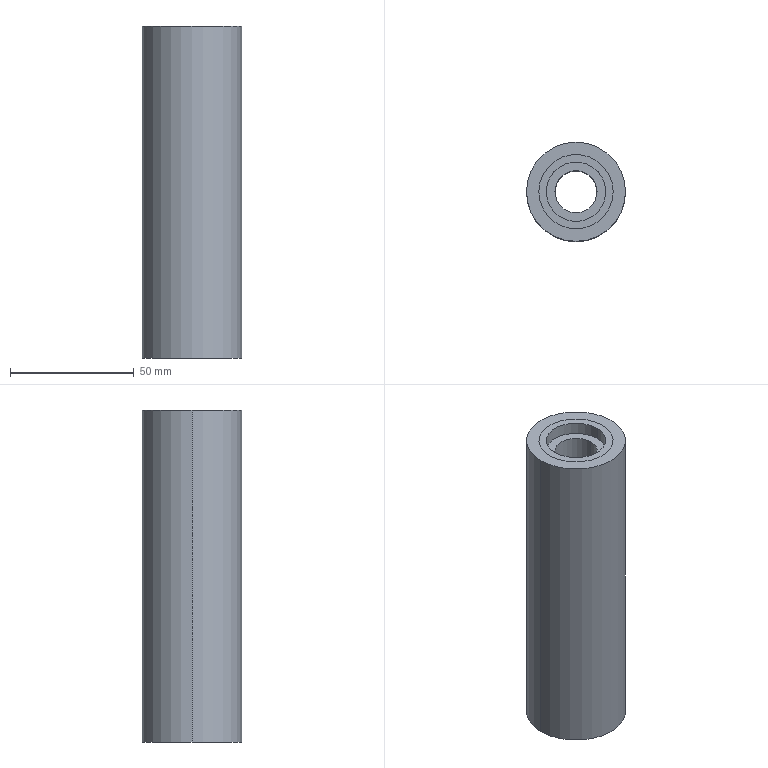Part | STEP file | MT-COMBO-119-S016 | 2 solids | 18 faces | box 40 x 40 x 134 mm | volume 135720 mm3 | cylinder 12 | plane 6 | commonest cylinder face diameters 24 x4 30 x4 17 x2 40 x2
STEP:
#1=CARTESIAN_POINT('',(12.,0.,62.));
#2=VERTEX_POINT('',#1);
#3=CARTESIAN_POINT('',(-12.,0.,62.));
#4=VERTEX_POINT('',#3);
#5=CARTESIAN_POINT('',(0.,0.,62.));
#6=DIRECTION('',(0.,0.,1.));
#7=DIRECTION('',(1.,0.,0.));
#8=AXIS2_PLACEMENT_3D('',#5,#6,#7);
#9=CIRCLE('',#8,12.);
#10=EDGE_CURVE('',#2,#4,#9,.T.);
#11=ORIENTED_EDGE('',*,*,#10,.F.);
#12=CARTESIAN_POINT('',(12.,0.,67.));
#13=VERTEX_POINT('',#12);
#14=CARTESIAN_POINT('',(12.,0.,62.));
#15=DIRECTION('',(0.,0.,1.));
#16=VECTOR('',#15,1000.);
#17=LINE('',#14,#16);
#18=EDGE_CURVE('',#2,#13,#17,.T.);
#19=ORIENTED_EDGE('',*,*,#18,.T.);
#20=CARTESIAN_POINT('',(-12.,0.,67.));
#21=VERTEX_POINT('',#20);
#22=CARTESIAN_POINT('',(0.,0.,67.));
#23=DIRECTION('',(0.,0.,1.));
#24=DIRECTION('',(1.,0.,0.));
#25=AXIS2_PLACEMENT_3D('',#22,#23,#24);
#26=CIRCLE('',#25,12.);
#27=EDGE_CURVE('',#13,#21,#26,.T.);
#28=ORIENTED_EDGE('',*,*,#27,.T.);
#29=CARTESIAN_POINT('',(-12.,0.,62.));
#30=DIRECTION('',(0.,0.,1.));
#31=VECTOR('',#30,1000.);
#32=LINE('',#29,#31);
#33=EDGE_CURVE('',#4,#21,#32,.T.);
#34=ORIENTED_EDGE('',*,*,#33,.F.);
#35=EDGE_LOOP('',(#11,#19,#28,#34));
#36=FACE_OUTER_BOUND('',#35,.T.);
#37=CARTESIAN_POINT('',(0.,0.,62.));
#38=DIRECTION('',(0.,0.,1.));
#39=DIRECTION('',(-1.,0.,0.));
#40=AXIS2_PLACEMENT_3D('',#37,#38,#39);
#41=CYLINDRICAL_SURFACE('',#40,12.);
#42=ADVANCED_FACE('',(#36),#41,.F.);
#43=CARTESIAN_POINT('',(12.,0.,-62.));
#44=VERTEX_POINT('',#43);
#45=CARTESIAN_POINT('',(-12.,0.,-62.));
#46=VERTEX_POINT('',#45);
#47=CARTESIAN_POINT('',(0.,0.,-62.));
#48=DIRECTION('',(0.,0.,1.));
#49=DIRECTION('',(1.,0.,0.));
#50=AXIS2_PLACEMENT_3D('',#47,#48,#49);
#51=CIRCLE('',#50,12.);
#52=EDGE_CURVE('',#44,#46,#51,.T.);
#53=ORIENTED_EDGE('',*,*,#52,.T.);
#54=CARTESIAN_POINT('',(-12.,0.,-67.));
#55=VERTEX_POINT('',#54);
#56=CARTESIAN_POINT('',(-12.,0.,-62.));
#57=DIRECTION('',(0.,0.,-1.));
#58=VECTOR('',#57,1000.);
#59=LINE('',#56,#58);
#60=EDGE_CURVE('',#46,#55,#59,.T.);
#61=ORIENTED_EDGE('',*,*,#60,.T.);
#62=CARTESIAN_POINT('',(12.,0.,-67.));
#63=VERTEX_POINT('',#62);
#64=CARTESIAN_POINT('',(0.,0.,-67.));
#65=DIRECTION('',(0.,0.,1.));
#66=DIRECTION('',(1.,0.,0.));
#67=AXIS2_PLACEMENT_3D('',#64,#65,#66);
#68=CIRCLE('',#67,12.);
#69=EDGE_CURVE('',#63,#55,#68,.T.);
#70=ORIENTED_EDGE('',*,*,#69,.F.);
#71=CARTESIAN_POINT('',(12.,0.,-62.));
#72=DIRECTION('',(0.,0.,-1.));
#73=VECTOR('',#72,1000.);
#74=LINE('',#71,#73);
#75=EDGE_CURVE('',#44,#63,#74,.T.);
#76=ORIENTED_EDGE('',*,*,#75,.F.);
#77=EDGE_LOOP('',(#53,#61,#70,#76));
#78=FACE_OUTER_BOUND('',#77,.T.);
#79=CARTESIAN_POINT('',(0.,0.,-62.));
#80=DIRECTION('',(0.,0.,-1.));
#81=DIRECTION('',(1.,0.,0.));
#82=AXIS2_PLACEMENT_3D('',#79,#80,#81);
#83=CYLINDRICAL_SURFACE('',#82,12.);
#84=ADVANCED_FACE('',(#78),#83,.F.);
#85=CARTESIAN_POINT('',(-15.,0.,-67.));
#86=VERTEX_POINT('',#85);
#87=CARTESIAN_POINT('',(15.,0.,-67.));
#88=VERTEX_POINT('',#87);
#89=CARTESIAN_POINT('',(0.,0.,-67.));
#90=DIRECTION('',(0.,0.,1.));
#91=DIRECTION('',(1.,0.,0.));
#92=AXIS2_PLACEMENT_3D('',#89,#90,#91);
#93=CIRCLE('',#92,15.);
#94=EDGE_CURVE('',#86,#88,#93,.T.);
#95=ORIENTED_EDGE('',*,*,#94,.T.);
#96=CARTESIAN_POINT('',(15.,0.,67.));
#97=VERTEX_POINT('',#96);
#98=CARTESIAN_POINT('',(15.,0.,-67.));
#99=DIRECTION('',(0.,0.,1.));
#100=VECTOR('',#99,1000.);
#101=LINE('',#98,#100);
#102=EDGE_CURVE('',#88,#97,#101,.T.);
#103=ORIENTED_EDGE('',*,*,#102,.T.);
#104=CARTESIAN_POINT('',(-15.,0.,67.));
#105=VERTEX_POINT('',#104);
#106=CARTESIAN_POINT('',(0.,0.,67.));
#107=DIRECTION('',(0.,0.,1.));
#108=DIRECTION('',(1.,0.,0.));
#109=AXIS2_PLACEMENT_3D('',#106,#107,#108);
#110=CIRCLE('',#109,15.);
#111=EDGE_CURVE('',#105,#97,#110,.T.);
#112=ORIENTED_EDGE('',*,*,#111,.F.);
#113=CARTESIAN_POINT('',(-15.,0.,-67.));
#114=DIRECTION('',(0.,0.,1.));
#115=VECTOR('',#114,1000.);
#116=LINE('',#113,#115);
#117=EDGE_CURVE('',#86,#105,#116,.T.);
#118=ORIENTED_EDGE('',*,*,#117,.F.);
#119=EDGE_LOOP('',(#95,#103,#112,#118));
#120=FACE_OUTER_BOUND('',#119,.T.);
#121=CARTESIAN_POINT('',(0.,0.,-67.));
#122=DIRECTION('',(0.,0.,1.));
#123=DIRECTION('',(-1.,0.,0.));
#124=AXIS2_PLACEMENT_3D('',#121,#122,#123);
#125=CYLINDRICAL_SURFACE('',#124,15.);
#126=ADVANCED_FACE('',(#120),#125,.T.);
#127=CARTESIAN_POINT('',(8.5,0.,-62.));
#128=VERTEX_POINT('',#127);
#129=CARTESIAN_POINT('',(-8.5,0.,-62.));
#130=VERTEX_POINT('',#129);
#131=CARTESIAN_POINT('',(0.,0.,-62.));
#132=DIRECTION('',(0.,0.,1.));
#133=DIRECTION('',(1.,0.,0.));
#134=AXIS2_PLACEMENT_3D('',#131,#132,#133);
#135=CIRCLE('',#134,8.5);
#136=EDGE_CURVE('',#128,#130,#135,.T.);
#137=ORIENTED_EDGE('',*,*,#136,.F.);
#138=CARTESIAN_POINT('',(8.5,0.,62.));
#139=VERTEX_POINT('',#138);
#140=CARTESIAN_POINT('',(8.5,0.,-67.));
#141=DIRECTION('',(0.,0.,1.));
#142=VECTOR('',#141,1000.);
#143=LINE('',#140,#142);
#144=EDGE_CURVE('',#128,#139,#143,.T.);
#145=ORIENTED_EDGE('',*,*,#144,.T.);
#146=CARTESIAN_POINT('',(-8.5,0.,62.));
#147=VERTEX_POINT('',#146);
#148=CARTESIAN_POINT('',(0.,0.,62.));
#149=DIRECTION('',(0.,0.,-1.));
#150=DIRECTION('',(-1.,0.,0.));
#151=AXIS2_PLACEMENT_3D('',#148,#149,#150);
#152=CIRCLE('',#151,8.5);
#153=EDGE_CURVE('',#147,#139,#152,.T.);
#154=ORIENTED_EDGE('',*,*,#153,.F.);
#155=CARTESIAN_POINT('',(-8.5,0.,-67.));
#156=DIRECTION('',(0.,0.,1.));
#157=VECTOR('',#156,1000.);
#158=LINE('',#155,#157);
#159=EDGE_CURVE('',#130,#147,#158,.T.);
#160=ORIENTED_EDGE('',*,*,#159,.F.);
#161=EDGE_LOOP('',(#137,#145,#154,#160));
#162=FACE_OUTER_BOUND('',#161,.T.);
#163=CARTESIAN_POINT('',(0.,0.,-67.));
#164=DIRECTION('',(0.,0.,1.));
#165=DIRECTION('',(-1.,0.,0.));
#166=AXIS2_PLACEMENT_3D('',#163,#164,#165);
#167=CYLINDRICAL_SURFACE('',#166,8.5);
#168=ADVANCED_FACE('',(#162),#167,.F.);
#169=ORIENTED_EDGE('',*,*,#144,.F.);
#170=CARTESIAN_POINT('',(0.,0.,-62.));
#171=DIRECTION('',(0.,0.,1.));
#172=DIRECTION('',(1.,0.,0.));
#173=AXIS2_PLACEMENT_3D('',#170,#171,#172);
#174=CIRCLE('',#173,8.5);
#175=EDGE_CURVE('',#130,#128,#174,.T.);
#176=ORIENTED_EDGE('',*,*,#175,.F.);
#177=ORIENTED_EDGE('',*,*,#159,.T.);
#178=CARTESIAN_POINT('',(0.,0.,62.));
#179=DIRECTION('',(0.,0.,-1.));
#180=DIRECTION('',(-1.,0.,0.));
#181=AXIS2_PLACEMENT_3D('',#178,#179,#180);
#182=CIRCLE('',#181,8.5);
#183=EDGE_CURVE('',#139,#147,#182,.T.);
#184=ORIENTED_EDGE('',*,*,#183,.F.);
#185=EDGE_LOOP('',(#169,#176,#177,#184));
#186=FACE_OUTER_BOUND('',#185,.T.);
#187=CARTESIAN_POINT('',(0.,0.,-67.));
#188=DIRECTION('',(0.,0.,1.));
#189=DIRECTION('',(-1.,0.,0.));
#190=AXIS2_PLACEMENT_3D('',#187,#188,#189);
#191=CYLINDRICAL_SURFACE('',#190,8.5);
#192=ADVANCED_FACE('',(#186),#191,.F.);
#193=ORIENTED_EDGE('',*,*,#69,.T.);
#194=CARTESIAN_POINT('',(0.,0.,-67.));
#195=DIRECTION('',(0.,0.,1.));
#196=DIRECTION('',(1.,0.,0.));
#197=AXIS2_PLACEMENT_3D('',#194,#195,#196);
#198=CIRCLE('',#197,12.);
#199=EDGE_CURVE('',#55,#63,#198,.T.);
#200=ORIENTED_EDGE('',*,*,#199,.T.);
#201=EDGE_LOOP('',(#193,#200));
#202=FACE_BOUND('',#201,.T.);
#203=ORIENTED_EDGE('',*,*,#94,.F.);
#204=CARTESIAN_POINT('',(0.,0.,-67.));
#205=DIRECTION('',(0.,0.,1.));
#206=DIRECTION('',(1.,0.,0.));
#207=AXIS2_PLACEMENT_3D('',#204,#205,#206);
#208=CIRCLE('',#207,15.);
#209=EDGE_CURVE('',#88,#86,#208,.T.);
#210=ORIENTED_EDGE('',*,*,#209,.F.);
#211=EDGE_LOOP('',(#203,#210));
#212=FACE_OUTER_BOUND('',#211,.T.);
#213=CARTESIAN_POINT('',(0.,0.,-67.));
#214=DIRECTION('',(0.,0.,-1.));
#215=DIRECTION('',(1.,0.,0.));
#216=AXIS2_PLACEMENT_3D('',#213,#214,#215);
#217=PLANE('',#216);
#218=ADVANCED_FACE('',(#202,#212),#217,.T.);
#219=CARTESIAN_POINT('',(0.,0.,67.));
#220=DIRECTION('',(0.,0.,1.));
#221=DIRECTION('',(1.,0.,0.));
#222=AXIS2_PLACEMENT_3D('',#219,#220,#221);
#223=CIRCLE('',#222,12.);
#224=EDGE_CURVE('',#21,#13,#223,.T.);
#225=ORIENTED_EDGE('',*,*,#224,.F.);
#226=ORIENTED_EDGE('',*,*,#27,.F.);
#227=EDGE_LOOP('',(#225,#226));
#228=FACE_BOUND('',#227,.T.);
#229=ORIENTED_EDGE('',*,*,#111,.T.);
#230=CARTESIAN_POINT('',(0.,0.,67.));
#231=DIRECTION('',(0.,0.,1.));
#232=DIRECTION('',(1.,0.,0.));
#233=AXIS2_PLACEMENT_3D('',#230,#231,#232);
#234=CIRCLE('',#233,15.);
#235=EDGE_CURVE('',#97,#105,#234,.T.);
#236=ORIENTED_EDGE('',*,*,#235,.T.);
#237=EDGE_LOOP('',(#229,#236));
#238=FACE_OUTER_BOUND('',#237,.T.);
#239=CARTESIAN_POINT('',(0.,0.,67.));
#240=DIRECTION('',(0.,0.,-1.));
#241=DIRECTION('',(1.,0.,0.));
#242=AXIS2_PLACEMENT_3D('',#239,#240,#241);
#243=PLANE('',#242);
#244=ADVANCED_FACE('',(#228,#238),#243,.F.);
#245=ORIENTED_EDGE('',*,*,#102,.F.);
#246=ORIENTED_EDGE('',*,*,#209,.T.);
#247=ORIENTED_EDGE('',*,*,#117,.T.);
#248=ORIENTED_EDGE('',*,*,#235,.F.);
#249=EDGE_LOOP('',(#245,#246,#247,#248));
#250=FACE_OUTER_BOUND('',#249,.T.);
#251=CARTESIAN_POINT('',(0.,0.,-67.));
#252=DIRECTION('',(0.,0.,1.));
#253=DIRECTION('',(-1.,0.,0.));
#254=AXIS2_PLACEMENT_3D('',#251,#252,#253);
#255=CYLINDRICAL_SURFACE('',#254,15.);
#256=ADVANCED_FACE('',(#250),#255,.T.);
#257=ORIENTED_EDGE('',*,*,#60,.F.);
#258=CARTESIAN_POINT('',(0.,0.,-62.));
#259=DIRECTION('',(0.,0.,1.));
#260=DIRECTION('',(1.,0.,0.));
#261=AXIS2_PLACEMENT_3D('',#258,#259,#260);
#262=CIRCLE('',#261,12.);
#263=EDGE_CURVE('',#46,#44,#262,.T.);
#264=ORIENTED_EDGE('',*,*,#263,.T.);
#265=ORIENTED_EDGE('',*,*,#75,.T.);
#266=ORIENTED_EDGE('',*,*,#199,.F.);
#267=EDGE_LOOP('',(#257,#264,#265,#266));
#268=FACE_OUTER_BOUND('',#267,.T.);
#269=CARTESIAN_POINT('',(0.,0.,-62.));
#270=DIRECTION('',(0.,0.,-1.));
#271=DIRECTION('',(1.,0.,0.));
#272=AXIS2_PLACEMENT_3D('',#269,#270,#271);
#273=CYLINDRICAL_SURFACE('',#272,12.);
#274=ADVANCED_FACE('',(#268),#273,.F.);
#275=ORIENTED_EDGE('',*,*,#175,.T.);
#276=ORIENTED_EDGE('',*,*,#136,.T.);
#277=EDGE_LOOP('',(#275,#276));
#278=FACE_BOUND('',#277,.T.);
#279=ORIENTED_EDGE('',*,*,#52,.F.);
#280=ORIENTED_EDGE('',*,*,#263,.F.);
#281=EDGE_LOOP('',(#279,#280));
#282=FACE_OUTER_BOUND('',#281,.T.);
#283=CARTESIAN_POINT('',(0.,0.,-62.));
#284=DIRECTION('',(0.,0.,-1.));
#285=DIRECTION('',(1.,0.,0.));
#286=AXIS2_PLACEMENT_3D('',#283,#284,#285);
#287=PLANE('',#286);
#288=ADVANCED_FACE('',(#278,#282),#287,.T.);
#289=ORIENTED_EDGE('',*,*,#18,.F.);
#290=CARTESIAN_POINT('',(0.,0.,62.));
#291=DIRECTION('',(0.,0.,1.));
#292=DIRECTION('',(1.,0.,0.));
#293=AXIS2_PLACEMENT_3D('',#290,#291,#292);
#294=CIRCLE('',#293,12.);
#295=EDGE_CURVE('',#4,#2,#294,.T.);
#296=ORIENTED_EDGE('',*,*,#295,.F.);
#297=ORIENTED_EDGE('',*,*,#33,.T.);
#298=ORIENTED_EDGE('',*,*,#224,.T.);
#299=EDGE_LOOP('',(#289,#296,#297,#298));
#300=FACE_OUTER_BOUND('',#299,.T.);
#301=CARTESIAN_POINT('',(0.,0.,62.));
#302=DIRECTION('',(0.,0.,1.));
#303=DIRECTION('',(-1.,0.,0.));
#304=AXIS2_PLACEMENT_3D('',#301,#302,#303);
#305=CYLINDRICAL_SURFACE('',#304,12.);
#306=ADVANCED_FACE('',(#300),#305,.F.);
#307=ORIENTED_EDGE('',*,*,#153,.T.);
#308=ORIENTED_EDGE('',*,*,#183,.T.);
#309=EDGE_LOOP('',(#307,#308));
#310=FACE_BOUND('',#309,.T.);
#311=ORIENTED_EDGE('',*,*,#295,.T.);
#312=ORIENTED_EDGE('',*,*,#10,.T.);
#313=EDGE_LOOP('',(#311,#312));
#314=FACE_OUTER_BOUND('',#313,.T.);
#315=CARTESIAN_POINT('',(0.,0.,62.));
#316=DIRECTION('',(0.,0.,1.));
#317=DIRECTION('',(1.,0.,0.));
#318=AXIS2_PLACEMENT_3D('',#315,#316,#317);
#319=PLANE('',#318);
#320=ADVANCED_FACE('',(#310,#314),#319,.T.);
#321=CLOSED_SHELL('',(#42,#84,#126,#168,#192,#218,#244,#256,#274,#288,#306,#320));
#322=MANIFOLD_SOLID_BREP('',#321);
#323=CARTESIAN_POINT('',(15.,0.,-67.));
#324=VERTEX_POINT('',#323);
#325=CARTESIAN_POINT('',(-15.,0.,-67.));
#326=VERTEX_POINT('',#325);
#327=CARTESIAN_POINT('',(0.,0.,-67.));
#328=DIRECTION('',(0.,0.,1.));
#329=DIRECTION('',(1.,0.,0.));
#330=AXIS2_PLACEMENT_3D('',#327,#328,#329);
#331=CIRCLE('',#330,15.);
#332=EDGE_CURVE('',#324,#326,#331,.T.);
#333=ORIENTED_EDGE('',*,*,#332,.F.);
#334=CARTESIAN_POINT('',(15.,0.,67.));
#335=VERTEX_POINT('',#334);
#336=CARTESIAN_POINT('',(15.,0.,-123.569));
#337=DIRECTION('',(0.,0.,1.));
#338=VECTOR('',#337,1000.);
#339=LINE('',#336,#338);
#340=EDGE_CURVE('',#324,#335,#339,.T.);
#341=ORIENTED_EDGE('',*,*,#340,.T.);
#342=CARTESIAN_POINT('',(-15.,0.,67.));
#343=VERTEX_POINT('',#342);
#344=CARTESIAN_POINT('',(0.,0.,67.));
#345=DIRECTION('',(0.,0.,-1.));
#346=DIRECTION('',(1.,0.,0.));
#347=AXIS2_PLACEMENT_3D('',#344,#345,#346);
#348=CIRCLE('',#347,15.);
#349=EDGE_CURVE('',#343,#335,#348,.T.);
#350=ORIENTED_EDGE('',*,*,#349,.F.);
#351=CARTESIAN_POINT('',(-15.,0.,-123.569));
#352=DIRECTION('',(0.,0.,1.));
#353=VECTOR('',#352,1000.);
#354=LINE('',#351,#353);
#355=EDGE_CURVE('',#326,#343,#354,.T.);
#356=ORIENTED_EDGE('',*,*,#355,.F.);
#357=EDGE_LOOP('',(#333,#341,#350,#356));
#358=FACE_OUTER_BOUND('',#357,.T.);
#359=CARTESIAN_POINT('',(0.,0.,-123.569));
#360=DIRECTION('',(0.,0.,1.));
#361=DIRECTION('',(-1.,0.,0.));
#362=AXIS2_PLACEMENT_3D('',#359,#360,#361);
#363=CYLINDRICAL_SURFACE('',#362,15.);
#364=ADVANCED_FACE('',(#358),#363,.F.);
#365=CARTESIAN_POINT('',(-20.,0.,-67.));
#366=VERTEX_POINT('',#365);
#367=CARTESIAN_POINT('',(20.,0.,-67.));
#368=VERTEX_POINT('',#367);
#369=CARTESIAN_POINT('',(0.,0.,-67.));
#370=DIRECTION('',(0.,0.,1.));
#371=DIRECTION('',(1.,0.,0.));
#372=AXIS2_PLACEMENT_3D('',#369,#370,#371);
#373=CIRCLE('',#372,20.);
#374=EDGE_CURVE('',#366,#368,#373,.T.);
#375=ORIENTED_EDGE('',*,*,#374,.T.);
#376=CARTESIAN_POINT('',(20.,0.,67.));
#377=VERTEX_POINT('',#376);
#378=CARTESIAN_POINT('',(20.,0.,-123.569));
#379=DIRECTION('',(0.,0.,1.));
#380=VECTOR('',#379,1000.);
#381=LINE('',#378,#380);
#382=EDGE_CURVE('',#368,#377,#381,.T.);
#383=ORIENTED_EDGE('',*,*,#382,.T.);
#384=CARTESIAN_POINT('',(-20.,0.,67.));
#385=VERTEX_POINT('',#384);
#386=CARTESIAN_POINT('',(0.,0.,67.));
#387=DIRECTION('',(0.,0.,-1.));
#388=DIRECTION('',(1.,0.,0.));
#389=AXIS2_PLACEMENT_3D('',#386,#387,#388);
#390=CIRCLE('',#389,20.);
#391=EDGE_CURVE('',#377,#385,#390,.T.);
#392=ORIENTED_EDGE('',*,*,#391,.T.);
#393=CARTESIAN_POINT('',(-20.,0.,-123.569));
#394=DIRECTION('',(0.,0.,1.));
#395=VECTOR('',#394,1000.);
#396=LINE('',#393,#395);
#397=EDGE_CURVE('',#366,#385,#396,.T.);
#398=ORIENTED_EDGE('',*,*,#397,.F.);
#399=EDGE_LOOP('',(#375,#383,#392,#398));
#400=FACE_OUTER_BOUND('',#399,.T.);
#401=CARTESIAN_POINT('',(0.,0.,-123.569));
#402=DIRECTION('',(0.,0.,1.));
#403=DIRECTION('',(-1.,0.,0.));
#404=AXIS2_PLACEMENT_3D('',#401,#402,#403);
#405=CYLINDRICAL_SURFACE('',#404,20.);
#406=ADVANCED_FACE('',(#400),#405,.T.);
#407=ORIENTED_EDGE('',*,*,#382,.F.);
#408=CARTESIAN_POINT('',(0.,0.,-67.));
#409=DIRECTION('',(0.,0.,1.));
#410=DIRECTION('',(1.,0.,0.));
#411=AXIS2_PLACEMENT_3D('',#408,#409,#410);
#412=CIRCLE('',#411,20.);
#413=EDGE_CURVE('',#368,#366,#412,.T.);
#414=ORIENTED_EDGE('',*,*,#413,.T.);
#415=ORIENTED_EDGE('',*,*,#397,.T.);
#416=CARTESIAN_POINT('',(0.,0.,67.));
#417=DIRECTION('',(0.,0.,-1.));
#418=DIRECTION('',(1.,0.,0.));
#419=AXIS2_PLACEMENT_3D('',#416,#417,#418);
#420=CIRCLE('',#419,20.);
#421=EDGE_CURVE('',#385,#377,#420,.T.);
#422=ORIENTED_EDGE('',*,*,#421,.T.);
#423=EDGE_LOOP('',(#407,#414,#415,#422));
#424=FACE_OUTER_BOUND('',#423,.T.);
#425=CARTESIAN_POINT('',(0.,0.,-123.569));
#426=DIRECTION('',(0.,0.,1.));
#427=DIRECTION('',(-1.,0.,0.));
#428=AXIS2_PLACEMENT_3D('',#425,#426,#427);
#429=CYLINDRICAL_SURFACE('',#428,20.);
#430=ADVANCED_FACE('',(#424),#429,.T.);
#431=ORIENTED_EDGE('',*,*,#340,.F.);
#432=CARTESIAN_POINT('',(0.,0.,-67.));
#433=DIRECTION('',(0.,0.,1.));
#434=DIRECTION('',(1.,0.,0.));
#435=AXIS2_PLACEMENT_3D('',#432,#433,#434);
#436=CIRCLE('',#435,15.);
#437=EDGE_CURVE('',#326,#324,#436,.T.);
#438=ORIENTED_EDGE('',*,*,#437,.F.);
#439=ORIENTED_EDGE('',*,*,#355,.T.);
#440=CARTESIAN_POINT('',(0.,0.,67.));
#441=DIRECTION('',(0.,0.,-1.));
#442=DIRECTION('',(1.,0.,0.));
#443=AXIS2_PLACEMENT_3D('',#440,#441,#442);
#444=CIRCLE('',#443,15.);
#445=EDGE_CURVE('',#335,#343,#444,.T.);
#446=ORIENTED_EDGE('',*,*,#445,.F.);
#447=EDGE_LOOP('',(#431,#438,#439,#446));
#448=FACE_OUTER_BOUND('',#447,.T.);
#449=CARTESIAN_POINT('',(0.,0.,-123.569));
#450=DIRECTION('',(0.,0.,1.));
#451=DIRECTION('',(-1.,0.,0.));
#452=AXIS2_PLACEMENT_3D('',#449,#450,#451);
#453=CYLINDRICAL_SURFACE('',#452,15.);
#454=ADVANCED_FACE('',(#448),#453,.F.);
#455=ORIENTED_EDGE('',*,*,#437,.T.);
#456=ORIENTED_EDGE('',*,*,#332,.T.);
#457=EDGE_LOOP('',(#455,#456));
#458=FACE_BOUND('',#457,.T.);
#459=ORIENTED_EDGE('',*,*,#374,.F.);
#460=ORIENTED_EDGE('',*,*,#413,.F.);
#461=EDGE_LOOP('',(#459,#460));
#462=FACE_OUTER_BOUND('',#461,.T.);
#463=CARTESIAN_POINT('',(0.,0.,-67.));
#464=DIRECTION('',(0.,0.,-1.));
#465=DIRECTION('',(1.,0.,0.));
#466=AXIS2_PLACEMENT_3D('',#463,#464,#465);
#467=PLANE('',#466);
#468=ADVANCED_FACE('',(#458,#462),#467,.T.);
#469=ORIENTED_EDGE('',*,*,#421,.F.);
#470=ORIENTED_EDGE('',*,*,#391,.F.);
#471=EDGE_LOOP('',(#469,#470));
#472=FACE_OUTER_BOUND('',#471,.T.);
#473=ORIENTED_EDGE('',*,*,#349,.T.);
#474=ORIENTED_EDGE('',*,*,#445,.T.);
#475=EDGE_LOOP('',(#473,#474));
#476=FACE_BOUND('',#475,.T.);
#477=CARTESIAN_POINT('',(0.,0.,67.));
#478=DIRECTION('',(0.,0.,-1.));
#479=DIRECTION('',(1.,0.,0.));
#480=AXIS2_PLACEMENT_3D('',#477,#478,#479);
#481=PLANE('',#480);
#482=ADVANCED_FACE('',(#472,#476),#481,.F.);
#483=CLOSED_SHELL('',(#364,#406,#430,#454,#468,#482));
#484=MANIFOLD_SOLID_BREP('',#483);
#485=CARTESIAN_POINT('',(0.,0.,0.));
#486=DIRECTION('',(0.,0.,1.));
#487=DIRECTION('',(1.,0.,0.));
#488=AXIS2_PLACEMENT_3D('',#485,#486,#487);
#489=(LENGTH_UNIT()NAMED_UNIT(*)SI_UNIT(.MILLI.,.METRE.));
#490=UNCERTAINTY_MEASURE_WITH_UNIT(LENGTH_MEASURE(0.00001),#489,'','');
#491=(NAMED_UNIT(*)PLANE_ANGLE_UNIT()SI_UNIT($,.RADIAN.));
#492=(NAMED_UNIT(*)SI_UNIT($,.STERADIAN.)SOLID_ANGLE_UNIT());
#493=(GEOMETRIC_REPRESENTATION_CONTEXT(3)GLOBAL_UNCERTAINTY_ASSIGNED_CONTEXT((#490))GLOBAL_UNIT_ASSIGNED_CONTEXT((#489,#491,#492))REPRESENTATION_CONTEXT('',''));
#494=ADVANCED_BREP_SHAPE_REPRESENTATION('',(#322,#484,#488),#493);